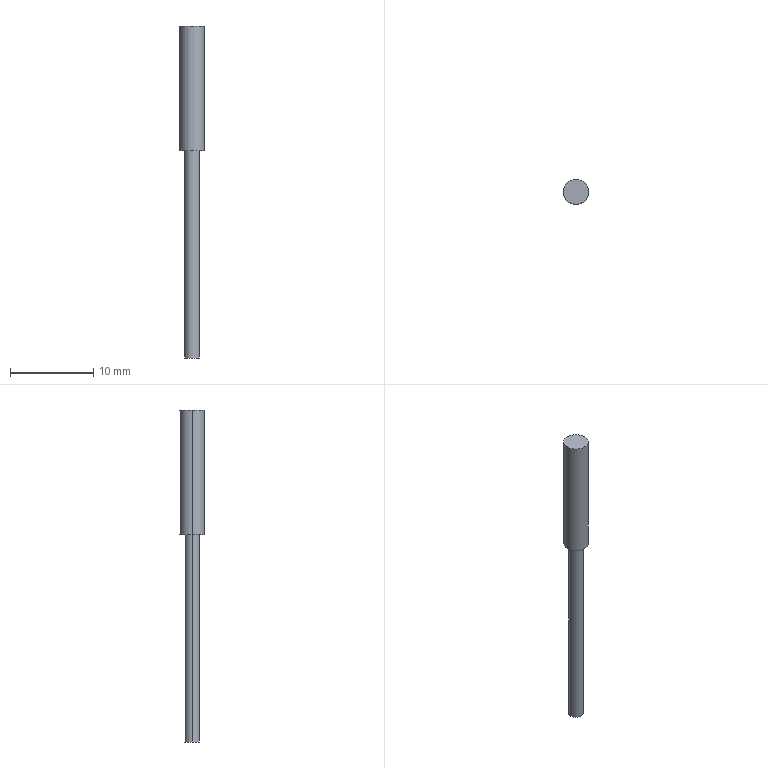Part | STEP file | E3X-HD10+E32-ZD200E | 1 solid | 7 faces | box 3 x 3 x 40 mm | volume 169.646 mm3 | cylinder 4 | plane 3 | commonest cylinder face diameters 1.8 x2 3 x2
STEP:
#1=CARTESIAN_POINT('',(0.,0.,0.));
#2=DIRECTION('',(0.,0.,1.));
#3=DIRECTION('',(1.,0.,0.));
#4=AXIS2_PLACEMENT_3D('',#1,#2,#3);
#5=CARTESIAN_POINT('',(-0.9,0.,-25.));
#6=VERTEX_POINT('',#5);
#7=CARTESIAN_POINT('',(0.9,0.,-25.));
#8=VERTEX_POINT('',#7);
#9=CARTESIAN_POINT('',(0.,0.,-25.));
#10=DIRECTION('',(0.,0.,-1.));
#11=DIRECTION('',(-1.,0.,0.));
#12=AXIS2_PLACEMENT_3D('',#9,#10,#11);
#13=CIRCLE('',#12,0.9);
#14=CARTESIAN_POINT('',(0.,0.,-25.));
#15=DIRECTION('',(0.,0.,1.));
#16=DIRECTION('',(1.,0.,0.));
#17=AXIS2_PLACEMENT_3D('',#14,#15,#16);
#18=CYLINDRICAL_SURFACE('',#17,0.9);
#19=CARTESIAN_POINT('',(3.142,0.));
#20=DIRECTION('',(-1.,0.));
#21=VECTOR('',#20,1.);
#22=LINE('',#19,#21);
#23=(GEOMETRIC_REPRESENTATION_CONTEXT(2)PARAMETRIC_REPRESENTATION_CONTEXT()REPRESENTATION_CONTEXT('',''));
#24=DEFINITIONAL_REPRESENTATION('',(#22),#23);
#25=PCURVE('',#18,#24);
#26=CARTESIAN_POINT('',(0.,0.,-25.));
#27=DIRECTION('',(0.,0.,-1.));
#28=DIRECTION('',(-1.,0.,0.));
#29=AXIS2_PLACEMENT_3D('',#26,#27,#28);
#30=PLANE('',#29);
#31=CARTESIAN_POINT('',(0.,0.));
#32=DIRECTION('',(1.,0.));
#33=AXIS2_PLACEMENT_2D('',#31,#32);
#34=CIRCLE('',#33,0.9);
#35=(GEOMETRIC_REPRESENTATION_CONTEXT(2)PARAMETRIC_REPRESENTATION_CONTEXT()REPRESENTATION_CONTEXT('',''));
#36=DEFINITIONAL_REPRESENTATION('',(#34),#35);
#37=PCURVE('',#30,#36);
#38=SURFACE_CURVE('',#13,(#25,#37),.PCURVE_S1.);
#39=EDGE_CURVE('',#6,#8,#38,.T.);
#40=ORIENTED_EDGE('',*,*,#39,.F.);
#41=CARTESIAN_POINT('',(-0.9,0.,0.));
#42=VERTEX_POINT('',#41);
#43=CARTESIAN_POINT('',(-0.9,0.,-25.));
#44=DIRECTION('',(0.,0.,1.));
#45=VECTOR('',#44,1.);
#46=LINE('',#43,#45);
#47=CARTESIAN_POINT('',(3.142,0.));
#48=DIRECTION('',(0.,1.));
#49=VECTOR('',#48,1.);
#50=LINE('',#47,#49);
#51=(GEOMETRIC_REPRESENTATION_CONTEXT(2)PARAMETRIC_REPRESENTATION_CONTEXT()REPRESENTATION_CONTEXT('',''));
#52=DEFINITIONAL_REPRESENTATION('',(#50),#51);
#53=PCURVE('',#18,#52);
#54=CARTESIAN_POINT('',(0.,0.,-25.));
#55=DIRECTION('',(0.,0.,1.));
#56=DIRECTION('',(1.,0.,0.));
#57=AXIS2_PLACEMENT_3D('',#54,#55,#56);
#58=CYLINDRICAL_SURFACE('',#57,0.9);
#59=CARTESIAN_POINT('',(3.142,0.));
#60=DIRECTION('',(0.,1.));
#61=VECTOR('',#60,1.);
#62=LINE('',#59,#61);
#63=(GEOMETRIC_REPRESENTATION_CONTEXT(2)PARAMETRIC_REPRESENTATION_CONTEXT()REPRESENTATION_CONTEXT('',''));
#64=DEFINITIONAL_REPRESENTATION('',(#62),#63);
#65=PCURVE('',#58,#64);
#66=SURFACE_CURVE('',#46,(#53,#65),.PCURVE_S1.);
#67=EDGE_CURVE('',#6,#42,#66,.T.);
#68=ORIENTED_EDGE('',*,*,#67,.T.);
#69=CARTESIAN_POINT('',(0.9,0.,0.));
#70=VERTEX_POINT('',#69);
#71=CARTESIAN_POINT('',(0.,0.,0.));
#72=DIRECTION('',(0.,0.,-1.));
#73=DIRECTION('',(1.,0.,0.));
#74=AXIS2_PLACEMENT_3D('',#71,#72,#73);
#75=CIRCLE('',#74,0.9);
#76=CARTESIAN_POINT('',(6.283,25.));
#77=DIRECTION('',(-1.,0.));
#78=VECTOR('',#77,1.);
#79=LINE('',#76,#78);
#80=(GEOMETRIC_REPRESENTATION_CONTEXT(2)PARAMETRIC_REPRESENTATION_CONTEXT()REPRESENTATION_CONTEXT('',''));
#81=DEFINITIONAL_REPRESENTATION('',(#79),#80);
#82=PCURVE('',#18,#81);
#83=CARTESIAN_POINT('',(0.,0.,0.));
#84=DIRECTION('',(0.,0.,1.));
#85=DIRECTION('',(1.,0.,0.));
#86=AXIS2_PLACEMENT_3D('',#83,#84,#85);
#87=PLANE('',#86);
#88=CARTESIAN_POINT('',(0.9,0.));
#89=CARTESIAN_POINT('',(0.9,-1.559));
#90=CARTESIAN_POINT('',(-0.45,-0.7794));
#91=CARTESIAN_POINT('',(-1.8,0.));
#92=CARTESIAN_POINT('',(-0.45,0.7794));
#93=CARTESIAN_POINT('',(0.9,1.559));
#94=CARTESIAN_POINT('',(0.9,0.));
#95=(BOUNDED_CURVE()B_SPLINE_CURVE(2,(#88,#89,#90,#91,#92,#93,#94),.UNSPECIFIED.,.T.,.F.)B_SPLINE_CURVE_WITH_KNOTS((1,2,2,2,2,1),(-2.094,0.,2.094,4.189,6.283,8.378),.UNSPECIFIED.)CURVE()GEOMETRIC_REPRESENTATION_ITEM()RATIONAL_B_SPLINE_CURVE((1.,0.5,1.,0.5,1.,0.5,1.))REPRESENTATION_ITEM(''));
#96=(GEOMETRIC_REPRESENTATION_CONTEXT(2)PARAMETRIC_REPRESENTATION_CONTEXT()REPRESENTATION_CONTEXT('',''));
#97=DEFINITIONAL_REPRESENTATION('',(#95),#96);
#98=PCURVE('',#87,#97);
#99=SURFACE_CURVE('',#75,(#82,#98),.PCURVE_S1.);
#100=EDGE_CURVE('',#42,#70,#99,.T.);
#101=ORIENTED_EDGE('',*,*,#100,.T.);
#102=CARTESIAN_POINT('',(0.9,0.,-25.));
#103=DIRECTION('',(0.,0.,1.));
#104=VECTOR('',#103,1.);
#105=LINE('',#102,#104);
#106=CARTESIAN_POINT('',(0.,0.));
#107=DIRECTION('',(0.,1.));
#108=VECTOR('',#107,1.);
#109=LINE('',#106,#108);
#110=(GEOMETRIC_REPRESENTATION_CONTEXT(2)PARAMETRIC_REPRESENTATION_CONTEXT()REPRESENTATION_CONTEXT('',''));
#111=DEFINITIONAL_REPRESENTATION('',(#109),#110);
#112=PCURVE('',#18,#111);
#113=CARTESIAN_POINT('',(6.283,0.));
#114=DIRECTION('',(0.,1.));
#115=VECTOR('',#114,1.);
#116=LINE('',#113,#115);
#117=(GEOMETRIC_REPRESENTATION_CONTEXT(2)PARAMETRIC_REPRESENTATION_CONTEXT()REPRESENTATION_CONTEXT('',''));
#118=DEFINITIONAL_REPRESENTATION('',(#116),#117);
#119=PCURVE('',#58,#118);
#120=SURFACE_CURVE('',#105,(#112,#119),.PCURVE_S1.);
#121=EDGE_CURVE('',#8,#70,#120,.T.);
#122=ORIENTED_EDGE('',*,*,#121,.F.);
#123=EDGE_LOOP('',(#40,#68,#101,#122));
#124=FACE_BOUND('',#123,.T.);
#125=ADVANCED_FACE('',(#124),#18,.T.);
#126=CARTESIAN_POINT('',(1.5,0.,15.));
#127=VERTEX_POINT('',#126);
#128=CARTESIAN_POINT('',(-1.5,0.,15.));
#129=VERTEX_POINT('',#128);
#130=CARTESIAN_POINT('',(0.,0.,15.));
#131=DIRECTION('',(0.,0.,1.));
#132=DIRECTION('',(1.,0.,0.));
#133=AXIS2_PLACEMENT_3D('',#130,#131,#132);
#134=CIRCLE('',#133,1.5);
#135=CARTESIAN_POINT('',(0.,0.,15.));
#136=DIRECTION('',(0.,0.,-1.));
#137=DIRECTION('',(-1.,0.,0.));
#138=AXIS2_PLACEMENT_3D('',#135,#136,#137);
#139=CYLINDRICAL_SURFACE('',#138,1.5);
#140=CARTESIAN_POINT('',(3.142,0.));
#141=DIRECTION('',(-1.,0.));
#142=VECTOR('',#141,1.);
#143=LINE('',#140,#142);
#144=(GEOMETRIC_REPRESENTATION_CONTEXT(2)PARAMETRIC_REPRESENTATION_CONTEXT()REPRESENTATION_CONTEXT('',''));
#145=DEFINITIONAL_REPRESENTATION('',(#143),#144);
#146=PCURVE('',#139,#145);
#147=CARTESIAN_POINT('',(0.,0.,15.));
#148=DIRECTION('',(0.,0.,1.));
#149=DIRECTION('',(1.,0.,0.));
#150=AXIS2_PLACEMENT_3D('',#147,#148,#149);
#151=PLANE('',#150);
#152=CARTESIAN_POINT('',(0.,0.));
#153=DIRECTION('',(1.,0.));
#154=AXIS2_PLACEMENT_2D('',#152,#153);
#155=CIRCLE('',#154,1.5);
#156=(GEOMETRIC_REPRESENTATION_CONTEXT(2)PARAMETRIC_REPRESENTATION_CONTEXT()REPRESENTATION_CONTEXT('',''));
#157=DEFINITIONAL_REPRESENTATION('',(#155),#156);
#158=PCURVE('',#151,#157);
#159=SURFACE_CURVE('',#134,(#146,#158),.PCURVE_S1.);
#160=EDGE_CURVE('',#127,#129,#159,.T.);
#161=ORIENTED_EDGE('',*,*,#160,.F.);
#162=CARTESIAN_POINT('',(1.5,0.,0.));
#163=VERTEX_POINT('',#162);
#164=CARTESIAN_POINT('',(1.5,0.,15.));
#165=DIRECTION('',(0.,0.,-1.));
#166=VECTOR('',#165,1.);
#167=LINE('',#164,#166);
#168=CARTESIAN_POINT('',(3.142,0.));
#169=DIRECTION('',(0.,1.));
#170=VECTOR('',#169,1.);
#171=LINE('',#168,#170);
#172=(GEOMETRIC_REPRESENTATION_CONTEXT(2)PARAMETRIC_REPRESENTATION_CONTEXT()REPRESENTATION_CONTEXT('',''));
#173=DEFINITIONAL_REPRESENTATION('',(#171),#172);
#174=PCURVE('',#139,#173);
#175=CARTESIAN_POINT('',(0.,0.,15.));
#176=DIRECTION('',(0.,0.,-1.));
#177=DIRECTION('',(-1.,0.,0.));
#178=AXIS2_PLACEMENT_3D('',#175,#176,#177);
#179=CYLINDRICAL_SURFACE('',#178,1.5);
#180=CARTESIAN_POINT('',(3.142,0.));
#181=DIRECTION('',(0.,1.));
#182=VECTOR('',#181,1.);
#183=LINE('',#180,#182);
#184=(GEOMETRIC_REPRESENTATION_CONTEXT(2)PARAMETRIC_REPRESENTATION_CONTEXT()REPRESENTATION_CONTEXT('',''));
#185=DEFINITIONAL_REPRESENTATION('',(#183),#184);
#186=PCURVE('',#179,#185);
#187=SURFACE_CURVE('',#167,(#174,#186),.PCURVE_S1.);
#188=EDGE_CURVE('',#127,#163,#187,.T.);
#189=ORIENTED_EDGE('',*,*,#188,.T.);
#190=CARTESIAN_POINT('',(-1.5,0.,0.));
#191=VERTEX_POINT('',#190);
#192=CARTESIAN_POINT('',(0.,0.,0.));
#193=DIRECTION('',(0.,0.,1.));
#194=DIRECTION('',(1.,0.,0.));
#195=AXIS2_PLACEMENT_3D('',#192,#193,#194);
#196=CIRCLE('',#195,1.5);
#197=CARTESIAN_POINT('',(3.142,15.));
#198=DIRECTION('',(-1.,0.));
#199=VECTOR('',#198,1.);
#200=LINE('',#197,#199);
#201=(GEOMETRIC_REPRESENTATION_CONTEXT(2)PARAMETRIC_REPRESENTATION_CONTEXT()REPRESENTATION_CONTEXT('',''));
#202=DEFINITIONAL_REPRESENTATION('',(#200),#201);
#203=PCURVE('',#139,#202);
#204=CARTESIAN_POINT('',(0.,0.));
#205=DIRECTION('',(1.,0.));
#206=AXIS2_PLACEMENT_2D('',#204,#205);
#207=CIRCLE('',#206,1.5);
#208=(GEOMETRIC_REPRESENTATION_CONTEXT(2)PARAMETRIC_REPRESENTATION_CONTEXT()REPRESENTATION_CONTEXT('',''));
#209=DEFINITIONAL_REPRESENTATION('',(#207),#208);
#210=PCURVE('',#87,#209);
#211=SURFACE_CURVE('',#196,(#203,#210),.PCURVE_S1.);
#212=EDGE_CURVE('',#163,#191,#211,.T.);
#213=ORIENTED_EDGE('',*,*,#212,.T.);
#214=CARTESIAN_POINT('',(-1.5,0.,15.));
#215=DIRECTION('',(0.,0.,-1.));
#216=VECTOR('',#215,1.);
#217=LINE('',#214,#216);
#218=CARTESIAN_POINT('',(0.,0.));
#219=DIRECTION('',(0.,1.));
#220=VECTOR('',#219,1.);
#221=LINE('',#218,#220);
#222=(GEOMETRIC_REPRESENTATION_CONTEXT(2)PARAMETRIC_REPRESENTATION_CONTEXT()REPRESENTATION_CONTEXT('',''));
#223=DEFINITIONAL_REPRESENTATION('',(#221),#222);
#224=PCURVE('',#139,#223);
#225=CARTESIAN_POINT('',(6.283,0.));
#226=DIRECTION('',(0.,1.));
#227=VECTOR('',#226,1.);
#228=LINE('',#225,#227);
#229=(GEOMETRIC_REPRESENTATION_CONTEXT(2)PARAMETRIC_REPRESENTATION_CONTEXT()REPRESENTATION_CONTEXT('',''));
#230=DEFINITIONAL_REPRESENTATION('',(#228),#229);
#231=PCURVE('',#179,#230);
#232=SURFACE_CURVE('',#217,(#224,#231),.PCURVE_S1.);
#233=EDGE_CURVE('',#129,#191,#232,.T.);
#234=ORIENTED_EDGE('',*,*,#233,.F.);
#235=EDGE_LOOP('',(#161,#189,#213,#234));
#236=FACE_BOUND('',#235,.T.);
#237=ADVANCED_FACE('',(#236),#139,.T.);
#238=CARTESIAN_POINT('',(0.,0.,0.));
#239=DIRECTION('',(0.,0.,1.));
#240=DIRECTION('',(1.,0.,0.));
#241=AXIS2_PLACEMENT_3D('',#238,#239,#240);
#242=CIRCLE('',#241,1.5);
#243=CARTESIAN_POINT('',(0.,0.));
#244=DIRECTION('',(1.,0.));
#245=AXIS2_PLACEMENT_2D('',#243,#244);
#246=CIRCLE('',#245,1.5);
#247=(GEOMETRIC_REPRESENTATION_CONTEXT(2)PARAMETRIC_REPRESENTATION_CONTEXT()REPRESENTATION_CONTEXT('',''));
#248=DEFINITIONAL_REPRESENTATION('',(#246),#247);
#249=PCURVE('',#87,#248);
#250=CARTESIAN_POINT('',(9.425,15.));
#251=DIRECTION('',(-1.,0.));
#252=VECTOR('',#251,1.);
#253=LINE('',#250,#252);
#254=(GEOMETRIC_REPRESENTATION_CONTEXT(2)PARAMETRIC_REPRESENTATION_CONTEXT()REPRESENTATION_CONTEXT('',''));
#255=DEFINITIONAL_REPRESENTATION('',(#253),#254);
#256=PCURVE('',#179,#255);
#257=SURFACE_CURVE('',#242,(#249,#256),.PCURVE_S1.);
#258=EDGE_CURVE('',#191,#163,#257,.T.);
#259=ORIENTED_EDGE('',*,*,#258,.F.);
#260=ORIENTED_EDGE('',*,*,#212,.F.);
#261=EDGE_LOOP('',(#259,#260));
#262=FACE_BOUND('',#261,.T.);
#263=CARTESIAN_POINT('',(0.,0.,0.));
#264=DIRECTION('',(0.,0.,-1.));
#265=DIRECTION('',(1.,0.,0.));
#266=AXIS2_PLACEMENT_3D('',#263,#264,#265);
#267=CIRCLE('',#266,0.9);
#268=CARTESIAN_POINT('',(0.9,0.));
#269=CARTESIAN_POINT('',(0.9,-1.559));
#270=CARTESIAN_POINT('',(-0.45,-0.7794));
#271=CARTESIAN_POINT('',(-1.8,0.));
#272=CARTESIAN_POINT('',(-0.45,0.7794));
#273=CARTESIAN_POINT('',(0.9,1.559));
#274=CARTESIAN_POINT('',(0.9,0.));
#275=(BOUNDED_CURVE()B_SPLINE_CURVE(2,(#268,#269,#270,#271,#272,#273,#274),.UNSPECIFIED.,.T.,.F.)B_SPLINE_CURVE_WITH_KNOTS((1,2,2,2,2,1),(-2.094,0.,2.094,4.189,6.283,8.378),.UNSPECIFIED.)CURVE()GEOMETRIC_REPRESENTATION_ITEM()RATIONAL_B_SPLINE_CURVE((1.,0.5,1.,0.5,1.,0.5,1.))REPRESENTATION_ITEM(''));
#276=(GEOMETRIC_REPRESENTATION_CONTEXT(2)PARAMETRIC_REPRESENTATION_CONTEXT()REPRESENTATION_CONTEXT('',''));
#277=DEFINITIONAL_REPRESENTATION('',(#275),#276);
#278=PCURVE('',#87,#277);
#279=CARTESIAN_POINT('',(6.283,25.));
#280=DIRECTION('',(-1.,0.));
#281=VECTOR('',#280,1.);
#282=LINE('',#279,#281);
#283=(GEOMETRIC_REPRESENTATION_CONTEXT(2)PARAMETRIC_REPRESENTATION_CONTEXT()REPRESENTATION_CONTEXT('',''));
#284=DEFINITIONAL_REPRESENTATION('',(#282),#283);
#285=PCURVE('',#58,#284);
#286=SURFACE_CURVE('',#267,(#278,#285),.PCURVE_S1.);
#287=EDGE_CURVE('',#70,#42,#286,.T.);
#288=ORIENTED_EDGE('',*,*,#287,.F.);
#289=ORIENTED_EDGE('',*,*,#100,.F.);
#290=EDGE_LOOP('',(#288,#289));
#291=FACE_BOUND('',#290,.T.);
#292=ADVANCED_FACE('',(#262,#291),#87,.F.);
#293=ORIENTED_EDGE('',*,*,#188,.F.);
#294=CARTESIAN_POINT('',(0.,0.,15.));
#295=DIRECTION('',(0.,0.,1.));
#296=DIRECTION('',(1.,0.,0.));
#297=AXIS2_PLACEMENT_3D('',#294,#295,#296);
#298=CIRCLE('',#297,1.5);
#299=CARTESIAN_POINT('',(9.425,0.));
#300=DIRECTION('',(-1.,0.));
#301=VECTOR('',#300,1.);
#302=LINE('',#299,#301);
#303=(GEOMETRIC_REPRESENTATION_CONTEXT(2)PARAMETRIC_REPRESENTATION_CONTEXT()REPRESENTATION_CONTEXT('',''));
#304=DEFINITIONAL_REPRESENTATION('',(#302),#303);
#305=PCURVE('',#179,#304);
#306=CARTESIAN_POINT('',(0.,0.));
#307=DIRECTION('',(1.,0.));
#308=AXIS2_PLACEMENT_2D('',#306,#307);
#309=CIRCLE('',#308,1.5);
#310=(GEOMETRIC_REPRESENTATION_CONTEXT(2)PARAMETRIC_REPRESENTATION_CONTEXT()REPRESENTATION_CONTEXT('',''));
#311=DEFINITIONAL_REPRESENTATION('',(#309),#310);
#312=PCURVE('',#151,#311);
#313=SURFACE_CURVE('',#298,(#305,#312),.PCURVE_S1.);
#314=EDGE_CURVE('',#129,#127,#313,.T.);
#315=ORIENTED_EDGE('',*,*,#314,.F.);
#316=ORIENTED_EDGE('',*,*,#233,.T.);
#317=ORIENTED_EDGE('',*,*,#258,.T.);
#318=EDGE_LOOP('',(#293,#315,#316,#317));
#319=FACE_BOUND('',#318,.T.);
#320=ADVANCED_FACE('',(#319),#179,.T.);
#321=ORIENTED_EDGE('',*,*,#314,.T.);
#322=ORIENTED_EDGE('',*,*,#160,.T.);
#323=EDGE_LOOP('',(#321,#322));
#324=FACE_BOUND('',#323,.T.);
#325=ADVANCED_FACE('',(#324),#151,.T.);
#326=ORIENTED_EDGE('',*,*,#67,.F.);
#327=CARTESIAN_POINT('',(0.,0.,-25.));
#328=DIRECTION('',(0.,0.,-1.));
#329=DIRECTION('',(-1.,0.,0.));
#330=AXIS2_PLACEMENT_3D('',#327,#328,#329);
#331=CIRCLE('',#330,0.9);
#332=CARTESIAN_POINT('',(9.425,0.));
#333=DIRECTION('',(-1.,0.));
#334=VECTOR('',#333,1.);
#335=LINE('',#332,#334);
#336=(GEOMETRIC_REPRESENTATION_CONTEXT(2)PARAMETRIC_REPRESENTATION_CONTEXT()REPRESENTATION_CONTEXT('',''));
#337=DEFINITIONAL_REPRESENTATION('',(#335),#336);
#338=PCURVE('',#58,#337);
#339=CARTESIAN_POINT('',(0.,0.));
#340=DIRECTION('',(1.,0.));
#341=AXIS2_PLACEMENT_2D('',#339,#340);
#342=CIRCLE('',#341,0.9);
#343=(GEOMETRIC_REPRESENTATION_CONTEXT(2)PARAMETRIC_REPRESENTATION_CONTEXT()REPRESENTATION_CONTEXT('',''));
#344=DEFINITIONAL_REPRESENTATION('',(#342),#343);
#345=PCURVE('',#30,#344);
#346=SURFACE_CURVE('',#331,(#338,#345),.PCURVE_S1.);
#347=EDGE_CURVE('',#8,#6,#346,.T.);
#348=ORIENTED_EDGE('',*,*,#347,.F.);
#349=ORIENTED_EDGE('',*,*,#121,.T.);
#350=ORIENTED_EDGE('',*,*,#287,.T.);
#351=EDGE_LOOP('',(#326,#348,#349,#350));
#352=FACE_BOUND('',#351,.T.);
#353=ADVANCED_FACE('',(#352),#58,.T.);
#354=ORIENTED_EDGE('',*,*,#347,.T.);
#355=ORIENTED_EDGE('',*,*,#39,.T.);
#356=EDGE_LOOP('',(#354,#355));
#357=FACE_BOUND('',#356,.T.);
#358=ADVANCED_FACE('',(#357),#30,.T.);
#359=CLOSED_SHELL('',(#125,#237,#292,#320,#325,#353,#358));
#360=MANIFOLD_SOLID_BREP('',#359);
#361=(LENGTH_UNIT()NAMED_UNIT(*)SI_UNIT(.MILLI.,.METRE.));
#362=UNCERTAINTY_MEASURE_WITH_UNIT(LENGTH_MEASURE(0.0000001),#361,'','');
#363=(NAMED_UNIT(*)PLANE_ANGLE_UNIT()SI_UNIT($,.RADIAN.));
#364=(NAMED_UNIT(*)SI_UNIT($,.STERADIAN.)SOLID_ANGLE_UNIT());
#365=(GEOMETRIC_REPRESENTATION_CONTEXT(3)GLOBAL_UNCERTAINTY_ASSIGNED_CONTEXT((#362))GLOBAL_UNIT_ASSIGNED_CONTEXT((#361,#363,#364))REPRESENTATION_CONTEXT('',''));
#366=ADVANCED_BREP_SHAPE_REPRESENTATION('',(#4,#360),#365);